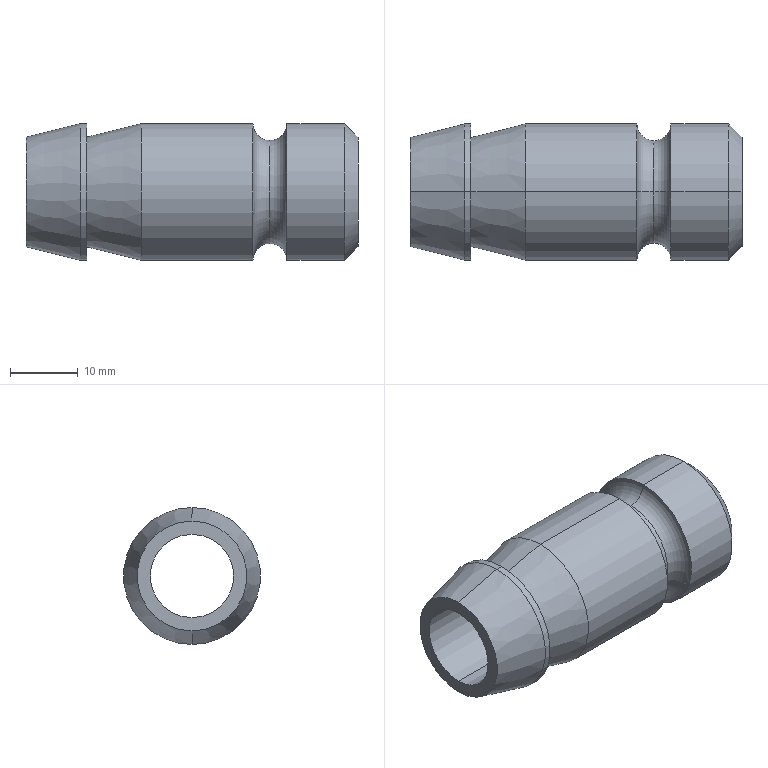Part | SolidWorks | features ICE 1, Revolution 1 | 1 solid | 21 faces | box 49 x 20.2 x 20.2 mm | volume 8256 mm3 | cylinder 8 | cone 6 | torus 4 | plane 3 | commonest cylinder face diameters 20.2 x6 12.3 x2
STEP:
#1=CARTESIAN_POINT('',(33.5,0.,10.1));
#2=VERTEX_POINT('',#1);
#3=CARTESIAN_POINT('',(36.,0.,7.6));
#4=VERTEX_POINT('',#3);
#5=CARTESIAN_POINT('',(36.,0.,10.1));
#6=DIRECTION('',(0.,-1.,0.));
#7=DIRECTION('',(0.,0.,-1.));
#8=AXIS2_PLACEMENT_3D('',#5,#6,#7);
#9=CIRCLE('',#8,2.5);
#10=EDGE_CURVE('',#2,#4,#9,.T.);
#11=ORIENTED_EDGE('',*,*,#10,.T.);
#12=CARTESIAN_POINT('',(36.,0.,-7.6));
#13=VERTEX_POINT('',#12);
#14=CARTESIAN_POINT('',(36.,0.,0.));
#15=DIRECTION('',(-1.,0.,0.));
#16=DIRECTION('',(0.,0.,1.));
#17=AXIS2_PLACEMENT_3D('',#14,#15,#16);
#18=CIRCLE('',#17,7.6);
#19=EDGE_CURVE('',#4,#13,#18,.T.);
#20=ORIENTED_EDGE('',*,*,#19,.T.);
#21=CARTESIAN_POINT('',(33.5,0.,-10.1));
#22=VERTEX_POINT('',#21);
#23=CARTESIAN_POINT('',(36.,0.,-10.1));
#24=DIRECTION('',(0.,1.,0.));
#25=DIRECTION('',(0.,0.,1.));
#26=AXIS2_PLACEMENT_3D('',#23,#24,#25);
#27=CIRCLE('',#26,2.5);
#28=EDGE_CURVE('',#22,#13,#27,.T.);
#29=ORIENTED_EDGE('',*,*,#28,.F.);
#30=CARTESIAN_POINT('',(33.5,0.,0.));
#31=DIRECTION('',(-1.,0.,0.));
#32=DIRECTION('',(0.,0.,1.));
#33=AXIS2_PLACEMENT_3D('',#30,#31,#32);
#34=CIRCLE('',#33,10.1);
#35=EDGE_CURVE('',#2,#22,#34,.T.);
#36=ORIENTED_EDGE('',*,*,#35,.F.);
#37=EDGE_LOOP('',(#11,#20,#29,#36));
#38=FACE_OUTER_BOUND('',#37,.T.);
#39=CARTESIAN_POINT('',(36.,0.,0.));
#40=DIRECTION('',(-1.,0.,0.));
#41=DIRECTION('',(0.,0.,1.));
#42=AXIS2_PLACEMENT_3D('',#39,#40,#41);
#43=TOROIDAL_SURFACE('',#42,10.1,2.5);
#44=ADVANCED_FACE('',(#38),#43,.F.);
#45=ORIENTED_EDGE('',*,*,#28,.T.);
#46=CARTESIAN_POINT('',(36.,0.,0.));
#47=DIRECTION('',(-1.,0.,0.));
#48=DIRECTION('',(0.,0.,1.));
#49=AXIS2_PLACEMENT_3D('',#46,#47,#48);
#50=CIRCLE('',#49,7.6);
#51=EDGE_CURVE('',#13,#4,#50,.T.);
#52=ORIENTED_EDGE('',*,*,#51,.T.);
#53=ORIENTED_EDGE('',*,*,#10,.F.);
#54=CARTESIAN_POINT('',(33.5,0.,0.));
#55=DIRECTION('',(-1.,0.,0.));
#56=DIRECTION('',(0.,0.,1.));
#57=AXIS2_PLACEMENT_3D('',#54,#55,#56);
#58=CIRCLE('',#57,10.1);
#59=EDGE_CURVE('',#22,#2,#58,.T.);
#60=ORIENTED_EDGE('',*,*,#59,.F.);
#61=EDGE_LOOP('',(#45,#52,#53,#60));
#62=FACE_OUTER_BOUND('',#61,.T.);
#63=CARTESIAN_POINT('',(36.,0.,0.));
#64=DIRECTION('',(-1.,0.,0.));
#65=DIRECTION('',(0.,0.,1.));
#66=AXIS2_PLACEMENT_3D('',#63,#64,#65);
#67=TOROIDAL_SURFACE('',#66,10.1,2.5);
#68=ADVANCED_FACE('',(#62),#67,.F.);
#69=CARTESIAN_POINT('',(49.,0.,-6.15));
#70=VERTEX_POINT('',#69);
#71=CARTESIAN_POINT('',(49.,0.,6.15));
#72=VERTEX_POINT('',#71);
#73=CARTESIAN_POINT('',(49.,0.,0.));
#74=DIRECTION('',(-1.,0.,0.));
#75=DIRECTION('',(0.,0.,1.));
#76=AXIS2_PLACEMENT_3D('',#73,#74,#75);
#77=CIRCLE('',#76,6.15);
#78=EDGE_CURVE('',#70,#72,#77,.T.);
#79=ORIENTED_EDGE('',*,*,#78,.F.);
#80=CARTESIAN_POINT('',(0.,0.,-6.15));
#81=VERTEX_POINT('',#80);
#82=CARTESIAN_POINT('',(99.,0.,-6.15));
#83=DIRECTION('',(-1.,0.,0.));
#84=VECTOR('',#83,1000.);
#85=LINE('',#82,#84);
#86=EDGE_CURVE('',#70,#81,#85,.T.);
#87=ORIENTED_EDGE('',*,*,#86,.T.);
#88=CARTESIAN_POINT('',(0.,0.,6.15));
#89=VERTEX_POINT('',#88);
#90=CARTESIAN_POINT('',(0.,0.,0.));
#91=DIRECTION('',(-1.,0.,0.));
#92=DIRECTION('',(0.,0.,1.));
#93=AXIS2_PLACEMENT_3D('',#90,#91,#92);
#94=CIRCLE('',#93,6.15);
#95=EDGE_CURVE('',#81,#89,#94,.T.);
#96=ORIENTED_EDGE('',*,*,#95,.T.);
#97=CARTESIAN_POINT('',(99.,0.,6.15));
#98=DIRECTION('',(-1.,0.,0.));
#99=VECTOR('',#98,1000.);
#100=LINE('',#97,#99);
#101=EDGE_CURVE('',#72,#89,#100,.T.);
#102=ORIENTED_EDGE('',*,*,#101,.F.);
#103=EDGE_LOOP('',(#79,#87,#96,#102));
#104=FACE_OUTER_BOUND('',#103,.T.);
#105=CARTESIAN_POINT('',(99.,0.,0.));
#106=DIRECTION('',(-1.,0.,0.));
#107=DIRECTION('',(0.,0.,1.));
#108=AXIS2_PLACEMENT_3D('',#105,#106,#107);
#109=CYLINDRICAL_SURFACE('',#108,6.15);
#110=ADVANCED_FACE('',(#104),#109,.F.);
#111=ORIENTED_EDGE('',*,*,#51,.F.);
#112=CARTESIAN_POINT('',(38.5,0.,-10.1));
#113=VERTEX_POINT('',#112);
#114=CARTESIAN_POINT('',(36.,0.,-10.1));
#115=DIRECTION('',(0.,1.,0.));
#116=DIRECTION('',(0.,0.,1.));
#117=AXIS2_PLACEMENT_3D('',#114,#115,#116);
#118=CIRCLE('',#117,2.5);
#119=EDGE_CURVE('',#13,#113,#118,.T.);
#120=ORIENTED_EDGE('',*,*,#119,.T.);
#121=CARTESIAN_POINT('',(38.5,0.,10.1));
#122=VERTEX_POINT('',#121);
#123=CARTESIAN_POINT('',(38.5,0.,0.));
#124=DIRECTION('',(-1.,0.,0.));
#125=DIRECTION('',(0.,0.,1.));
#126=AXIS2_PLACEMENT_3D('',#123,#124,#125);
#127=CIRCLE('',#126,10.1);
#128=EDGE_CURVE('',#113,#122,#127,.T.);
#129=ORIENTED_EDGE('',*,*,#128,.T.);
#130=CARTESIAN_POINT('',(36.,0.,10.1));
#131=DIRECTION('',(0.,-1.,0.));
#132=DIRECTION('',(0.,0.,-1.));
#133=AXIS2_PLACEMENT_3D('',#130,#131,#132);
#134=CIRCLE('',#133,2.5);
#135=EDGE_CURVE('',#4,#122,#134,.T.);
#136=ORIENTED_EDGE('',*,*,#135,.F.);
#137=EDGE_LOOP('',(#111,#120,#129,#136));
#138=FACE_OUTER_BOUND('',#137,.T.);
#139=CARTESIAN_POINT('',(36.,0.,0.));
#140=DIRECTION('',(-1.,0.,0.));
#141=DIRECTION('',(0.,0.,1.));
#142=AXIS2_PLACEMENT_3D('',#139,#140,#141);
#143=TOROIDAL_SURFACE('',#142,10.1,2.5);
#144=ADVANCED_FACE('',(#138),#143,.F.);
#145=CARTESIAN_POINT('',(47.,0.,10.1));
#146=VERTEX_POINT('',#145);
#147=CARTESIAN_POINT('',(47.,0.,-10.1));
#148=VERTEX_POINT('',#147);
#149=CARTESIAN_POINT('',(47.,0.,0.));
#150=DIRECTION('',(-1.,0.,0.));
#151=DIRECTION('',(0.,0.,1.));
#152=AXIS2_PLACEMENT_3D('',#149,#150,#151);
#153=CIRCLE('',#152,10.1);
#154=EDGE_CURVE('',#146,#148,#153,.T.);
#155=ORIENTED_EDGE('',*,*,#154,.T.);
#156=CARTESIAN_POINT('',(0.,0.,-10.1));
#157=DIRECTION('',(-1.,0.,0.));
#158=VECTOR('',#157,1000.);
#159=LINE('',#156,#158);
#160=EDGE_CURVE('',#148,#113,#159,.T.);
#161=ORIENTED_EDGE('',*,*,#160,.T.);
#162=CARTESIAN_POINT('',(38.5,0.,0.));
#163=DIRECTION('',(-1.,0.,0.));
#164=DIRECTION('',(0.,0.,1.));
#165=AXIS2_PLACEMENT_3D('',#162,#163,#164);
#166=CIRCLE('',#165,10.1);
#167=EDGE_CURVE('',#122,#113,#166,.T.);
#168=ORIENTED_EDGE('',*,*,#167,.F.);
#169=CARTESIAN_POINT('',(0.,0.,10.1));
#170=DIRECTION('',(-1.,0.,0.));
#171=VECTOR('',#170,1000.);
#172=LINE('',#169,#171);
#173=EDGE_CURVE('',#146,#122,#172,.T.);
#174=ORIENTED_EDGE('',*,*,#173,.F.);
#175=EDGE_LOOP('',(#155,#161,#168,#174));
#176=FACE_OUTER_BOUND('',#175,.T.);
#177=CARTESIAN_POINT('',(0.,0.,0.));
#178=DIRECTION('',(-1.,0.,0.));
#179=DIRECTION('',(0.,0.,1.));
#180=AXIS2_PLACEMENT_3D('',#177,#178,#179);
#181=CYLINDRICAL_SURFACE('',#180,10.1);
#182=ADVANCED_FACE('',(#176),#181,.T.);
#183=CARTESIAN_POINT('',(49.,0.,8.1));
#184=VERTEX_POINT('',#183);
#185=CARTESIAN_POINT('',(49.,0.,-8.1));
#186=VERTEX_POINT('',#185);
#187=CARTESIAN_POINT('',(49.,0.,0.));
#188=DIRECTION('',(-1.,0.,0.));
#189=DIRECTION('',(0.,0.,1.));
#190=AXIS2_PLACEMENT_3D('',#187,#188,#189);
#191=CIRCLE('',#190,8.1);
#192=EDGE_CURVE('',#184,#186,#191,.T.);
#193=ORIENTED_EDGE('',*,*,#192,.T.);
#194=CARTESIAN_POINT('',(49.,0.,-8.1));
#195=DIRECTION('',(-0.7071,0.,-0.7071));
#196=VECTOR('',#195,1000.);
#197=LINE('',#194,#196);
#198=EDGE_CURVE('',#186,#148,#197,.T.);
#199=ORIENTED_EDGE('',*,*,#198,.T.);
#200=ORIENTED_EDGE('',*,*,#154,.F.);
#201=CARTESIAN_POINT('',(49.,0.,8.1));
#202=DIRECTION('',(-0.7071,0.,0.7071));
#203=VECTOR('',#202,1000.);
#204=LINE('',#201,#203);
#205=EDGE_CURVE('',#184,#146,#204,.T.);
#206=ORIENTED_EDGE('',*,*,#205,.F.);
#207=EDGE_LOOP('',(#193,#199,#200,#206));
#208=FACE_OUTER_BOUND('',#207,.T.);
#209=CARTESIAN_POINT('',(49.,0.,0.));
#210=DIRECTION('',(-1.,0.,0.));
#211=DIRECTION('',(0.,0.,1.));
#212=AXIS2_PLACEMENT_3D('',#209,#210,#211);
#213=CONICAL_SURFACE('',#212,8.1,0.7854);
#214=ADVANCED_FACE('',(#208),#213,.T.);
#215=CARTESIAN_POINT('',(0.,0.,8.1));
#216=VERTEX_POINT('',#215);
#217=CARTESIAN_POINT('',(0.,0.,-8.1));
#218=VERTEX_POINT('',#217);
#219=CARTESIAN_POINT('',(0.,0.,0.));
#220=DIRECTION('',(-1.,0.,0.));
#221=DIRECTION('',(0.,0.,1.));
#222=AXIS2_PLACEMENT_3D('',#219,#220,#221);
#223=CIRCLE('',#222,8.1);
#224=EDGE_CURVE('',#216,#218,#223,.T.);
#225=ORIENTED_EDGE('',*,*,#224,.F.);
#226=CARTESIAN_POINT('',(8.,0.,10.1));
#227=VERTEX_POINT('',#226);
#228=CARTESIAN_POINT('',(8.,0.,10.1));
#229=DIRECTION('',(0.9701,0.,0.2425));
#230=VECTOR('',#229,1000.);
#231=LINE('',#228,#230);
#232=EDGE_CURVE('',#216,#227,#231,.T.);
#233=ORIENTED_EDGE('',*,*,#232,.T.);
#234=CARTESIAN_POINT('',(8.,0.,-10.1));
#235=VERTEX_POINT('',#234);
#236=CARTESIAN_POINT('',(8.,0.,0.));
#237=DIRECTION('',(-1.,0.,0.));
#238=DIRECTION('',(0.,0.,1.));
#239=AXIS2_PLACEMENT_3D('',#236,#237,#238);
#240=CIRCLE('',#239,10.1);
#241=EDGE_CURVE('',#227,#235,#240,.T.);
#242=ORIENTED_EDGE('',*,*,#241,.T.);
#243=CARTESIAN_POINT('',(8.,0.,-10.1));
#244=DIRECTION('',(0.9701,0.,-0.2425));
#245=VECTOR('',#244,1000.);
#246=LINE('',#243,#245);
#247=EDGE_CURVE('',#218,#235,#246,.T.);
#248=ORIENTED_EDGE('',*,*,#247,.F.);
#249=EDGE_LOOP('',(#225,#233,#242,#248));
#250=FACE_OUTER_BOUND('',#249,.T.);
#251=CARTESIAN_POINT('',(8.,0.,0.));
#252=DIRECTION('',(1.,0.,0.));
#253=DIRECTION('',(0.,0.,-1.));
#254=AXIS2_PLACEMENT_3D('',#251,#252,#253);
#255=CONICAL_SURFACE('',#254,10.1,0.245);
#256=ADVANCED_FACE('',(#250),#255,.T.);
#257=CARTESIAN_POINT('',(9.,0.,10.1));
#258=VERTEX_POINT('',#257);
#259=CARTESIAN_POINT('',(9.,0.,-10.1));
#260=VERTEX_POINT('',#259);
#261=CARTESIAN_POINT('',(9.,0.,0.));
#262=DIRECTION('',(-1.,0.,0.));
#263=DIRECTION('',(0.,0.,1.));
#264=AXIS2_PLACEMENT_3D('',#261,#262,#263);
#265=CIRCLE('',#264,10.1);
#266=EDGE_CURVE('',#258,#260,#265,.T.);
#267=ORIENTED_EDGE('',*,*,#266,.T.);
#268=CARTESIAN_POINT('',(0.,0.,-10.1));
#269=DIRECTION('',(-1.,0.,0.));
#270=VECTOR('',#269,1000.);
#271=LINE('',#268,#270);
#272=EDGE_CURVE('',#260,#235,#271,.T.);
#273=ORIENTED_EDGE('',*,*,#272,.T.);
#274=ORIENTED_EDGE('',*,*,#241,.F.);
#275=CARTESIAN_POINT('',(0.,0.,10.1));
#276=DIRECTION('',(-1.,0.,0.));
#277=VECTOR('',#276,1000.);
#278=LINE('',#275,#277);
#279=EDGE_CURVE('',#258,#227,#278,.T.);
#280=ORIENTED_EDGE('',*,*,#279,.F.);
#281=EDGE_LOOP('',(#267,#273,#274,#280));
#282=FACE_OUTER_BOUND('',#281,.T.);
#283=CARTESIAN_POINT('',(0.,0.,0.));
#284=DIRECTION('',(-1.,0.,0.));
#285=DIRECTION('',(0.,0.,1.));
#286=AXIS2_PLACEMENT_3D('',#283,#284,#285);
#287=CYLINDRICAL_SURFACE('',#286,10.1);
#288=ADVANCED_FACE('',(#282),#287,.T.);
#289=CARTESIAN_POINT('',(9.,0.,8.1));
#290=VERTEX_POINT('',#289);
#291=CARTESIAN_POINT('',(9.,0.,-8.1));
#292=VERTEX_POINT('',#291);
#293=CARTESIAN_POINT('',(9.,0.,0.));
#294=DIRECTION('',(-1.,0.,0.));
#295=DIRECTION('',(0.,0.,1.));
#296=AXIS2_PLACEMENT_3D('',#293,#294,#295);
#297=CIRCLE('',#296,8.1);
#298=EDGE_CURVE('',#290,#292,#297,.T.);
#299=ORIENTED_EDGE('',*,*,#298,.F.);
#300=CARTESIAN_POINT('',(17.,0.,10.1));
#301=VERTEX_POINT('',#300);
#302=CARTESIAN_POINT('',(17.,0.,10.1));
#303=DIRECTION('',(0.9701,0.,0.2425));
#304=VECTOR('',#303,1000.);
#305=LINE('',#302,#304);
#306=EDGE_CURVE('',#290,#301,#305,.T.);
#307=ORIENTED_EDGE('',*,*,#306,.T.);
#308=CARTESIAN_POINT('',(17.,0.,-10.1));
#309=VERTEX_POINT('',#308);
#310=CARTESIAN_POINT('',(17.,0.,0.));
#311=DIRECTION('',(-1.,0.,0.));
#312=DIRECTION('',(0.,0.,1.));
#313=AXIS2_PLACEMENT_3D('',#310,#311,#312);
#314=CIRCLE('',#313,10.1);
#315=EDGE_CURVE('',#301,#309,#314,.T.);
#316=ORIENTED_EDGE('',*,*,#315,.T.);
#317=CARTESIAN_POINT('',(17.,0.,-10.1));
#318=DIRECTION('',(0.9701,0.,-0.2425));
#319=VECTOR('',#318,1000.);
#320=LINE('',#317,#319);
#321=EDGE_CURVE('',#292,#309,#320,.T.);
#322=ORIENTED_EDGE('',*,*,#321,.F.);
#323=EDGE_LOOP('',(#299,#307,#316,#322));
#324=FACE_OUTER_BOUND('',#323,.T.);
#325=CARTESIAN_POINT('',(17.,0.,0.));
#326=DIRECTION('',(1.,0.,0.));
#327=DIRECTION('',(0.,0.,-1.));
#328=AXIS2_PLACEMENT_3D('',#325,#326,#327);
#329=CONICAL_SURFACE('',#328,10.1,0.245);
#330=ADVANCED_FACE('',(#324),#329,.T.);
#331=ORIENTED_EDGE('',*,*,#35,.T.);
#332=CARTESIAN_POINT('',(0.,0.,-10.1));
#333=DIRECTION('',(-1.,0.,0.));
#334=VECTOR('',#333,1000.);
#335=LINE('',#332,#334);
#336=EDGE_CURVE('',#22,#309,#335,.T.);
#337=ORIENTED_EDGE('',*,*,#336,.T.);
#338=ORIENTED_EDGE('',*,*,#315,.F.);
#339=CARTESIAN_POINT('',(0.,0.,10.1));
#340=DIRECTION('',(-1.,0.,0.));
#341=VECTOR('',#340,1000.);
#342=LINE('',#339,#341);
#343=EDGE_CURVE('',#2,#301,#342,.T.);
#344=ORIENTED_EDGE('',*,*,#343,.F.);
#345=EDGE_LOOP('',(#331,#337,#338,#344));
#346=FACE_OUTER_BOUND('',#345,.T.);
#347=CARTESIAN_POINT('',(0.,0.,0.));
#348=DIRECTION('',(-1.,0.,0.));
#349=DIRECTION('',(0.,0.,1.));
#350=AXIS2_PLACEMENT_3D('',#347,#348,#349);
#351=CYLINDRICAL_SURFACE('',#350,10.1);
#352=ADVANCED_FACE('',(#346),#351,.T.);
#353=ORIENTED_EDGE('',*,*,#336,.F.);
#354=ORIENTED_EDGE('',*,*,#59,.T.);
#355=ORIENTED_EDGE('',*,*,#343,.T.);
#356=CARTESIAN_POINT('',(17.,0.,0.));
#357=DIRECTION('',(-1.,0.,0.));
#358=DIRECTION('',(0.,0.,1.));
#359=AXIS2_PLACEMENT_3D('',#356,#357,#358);
#360=CIRCLE('',#359,10.1);
#361=EDGE_CURVE('',#309,#301,#360,.T.);
#362=ORIENTED_EDGE('',*,*,#361,.F.);
#363=EDGE_LOOP('',(#353,#354,#355,#362));
#364=FACE_OUTER_BOUND('',#363,.T.);
#365=CARTESIAN_POINT('',(0.,0.,0.));
#366=DIRECTION('',(-1.,0.,0.));
#367=DIRECTION('',(0.,0.,1.));
#368=AXIS2_PLACEMENT_3D('',#365,#366,#367);
#369=CYLINDRICAL_SURFACE('',#368,10.1);
#370=ADVANCED_FACE('',(#364),#369,.T.);
#371=ORIENTED_EDGE('',*,*,#306,.F.);
#372=CARTESIAN_POINT('',(9.,0.,0.));
#373=DIRECTION('',(-1.,0.,0.));
#374=DIRECTION('',(0.,0.,1.));
#375=AXIS2_PLACEMENT_3D('',#372,#373,#374);
#376=CIRCLE('',#375,8.1);
#377=EDGE_CURVE('',#292,#290,#376,.T.);
#378=ORIENTED_EDGE('',*,*,#377,.F.);
#379=ORIENTED_EDGE('',*,*,#321,.T.);
#380=ORIENTED_EDGE('',*,*,#361,.T.);
#381=EDGE_LOOP('',(#371,#378,#379,#380));
#382=FACE_OUTER_BOUND('',#381,.T.);
#383=CARTESIAN_POINT('',(17.,0.,0.));
#384=DIRECTION('',(1.,0.,0.));
#385=DIRECTION('',(0.,0.,-1.));
#386=AXIS2_PLACEMENT_3D('',#383,#384,#385);
#387=CONICAL_SURFACE('',#386,10.1,0.245);
#388=ADVANCED_FACE('',(#382),#387,.T.);
#389=ORIENTED_EDGE('',*,*,#266,.F.);
#390=CARTESIAN_POINT('',(9.,0.,0.));
#391=DIRECTION('',(-1.,0.,0.));
#392=DIRECTION('',(0.,0.,1.));
#393=AXIS2_PLACEMENT_3D('',#390,#391,#392);
#394=CIRCLE('',#393,10.1);
#395=EDGE_CURVE('',#260,#258,#394,.T.);
#396=ORIENTED_EDGE('',*,*,#395,.F.);
#397=EDGE_LOOP('',(#389,#396));
#398=FACE_OUTER_BOUND('',#397,.T.);
#399=ORIENTED_EDGE('',*,*,#377,.T.);
#400=ORIENTED_EDGE('',*,*,#298,.T.);
#401=EDGE_LOOP('',(#399,#400));
#402=FACE_BOUND('',#401,.T.);
#403=CARTESIAN_POINT('',(9.,8.1,0.));
#404=DIRECTION('',(-1.,0.,0.));
#405=DIRECTION('',(0.,0.,1.));
#406=AXIS2_PLACEMENT_3D('',#403,#404,#405);
#407=PLANE('',#406);
#408=ADVANCED_FACE('',(#398,#402),#407,.F.);
#409=ORIENTED_EDGE('',*,*,#272,.F.);
#410=ORIENTED_EDGE('',*,*,#395,.T.);
#411=ORIENTED_EDGE('',*,*,#279,.T.);
#412=CARTESIAN_POINT('',(8.,0.,0.));
#413=DIRECTION('',(-1.,0.,0.));
#414=DIRECTION('',(0.,0.,1.));
#415=AXIS2_PLACEMENT_3D('',#412,#413,#414);
#416=CIRCLE('',#415,10.1);
#417=EDGE_CURVE('',#235,#227,#416,.T.);
#418=ORIENTED_EDGE('',*,*,#417,.F.);
#419=EDGE_LOOP('',(#409,#410,#411,#418));
#420=FACE_OUTER_BOUND('',#419,.T.);
#421=CARTESIAN_POINT('',(0.,0.,0.));
#422=DIRECTION('',(-1.,0.,0.));
#423=DIRECTION('',(0.,0.,1.));
#424=AXIS2_PLACEMENT_3D('',#421,#422,#423);
#425=CYLINDRICAL_SURFACE('',#424,10.1);
#426=ADVANCED_FACE('',(#420),#425,.T.);
#427=ORIENTED_EDGE('',*,*,#232,.F.);
#428=CARTESIAN_POINT('',(0.,0.,0.));
#429=DIRECTION('',(-1.,0.,0.));
#430=DIRECTION('',(0.,0.,1.));
#431=AXIS2_PLACEMENT_3D('',#428,#429,#430);
#432=CIRCLE('',#431,8.1);
#433=EDGE_CURVE('',#218,#216,#432,.T.);
#434=ORIENTED_EDGE('',*,*,#433,.F.);
#435=ORIENTED_EDGE('',*,*,#247,.T.);
#436=ORIENTED_EDGE('',*,*,#417,.T.);
#437=EDGE_LOOP('',(#427,#434,#435,#436));
#438=FACE_OUTER_BOUND('',#437,.T.);
#439=CARTESIAN_POINT('',(8.,0.,0.));
#440=DIRECTION('',(1.,0.,0.));
#441=DIRECTION('',(0.,0.,-1.));
#442=AXIS2_PLACEMENT_3D('',#439,#440,#441);
#443=CONICAL_SURFACE('',#442,10.1,0.245);
#444=ADVANCED_FACE('',(#438),#443,.T.);
#445=CARTESIAN_POINT('',(0.,0.,0.));
#446=DIRECTION('',(-1.,0.,0.));
#447=DIRECTION('',(0.,0.,1.));
#448=AXIS2_PLACEMENT_3D('',#445,#446,#447);
#449=CIRCLE('',#448,6.15);
#450=EDGE_CURVE('',#89,#81,#449,.T.);
#451=ORIENTED_EDGE('',*,*,#450,.F.);
#452=ORIENTED_EDGE('',*,*,#95,.F.);
#453=EDGE_LOOP('',(#451,#452));
#454=FACE_BOUND('',#453,.T.);
#455=ORIENTED_EDGE('',*,*,#433,.T.);
#456=ORIENTED_EDGE('',*,*,#224,.T.);
#457=EDGE_LOOP('',(#455,#456));
#458=FACE_OUTER_BOUND('',#457,.T.);
#459=CARTESIAN_POINT('',(0.,8.1,0.));
#460=DIRECTION('',(1.,0.,0.));
#461=DIRECTION('',(0.,0.,-1.));
#462=AXIS2_PLACEMENT_3D('',#459,#460,#461);
#463=PLANE('',#462);
#464=ADVANCED_FACE('',(#454,#458),#463,.F.);
#465=CARTESIAN_POINT('',(49.,0.,0.));
#466=DIRECTION('',(-1.,0.,0.));
#467=DIRECTION('',(0.,0.,1.));
#468=AXIS2_PLACEMENT_3D('',#465,#466,#467);
#469=CIRCLE('',#468,6.15);
#470=EDGE_CURVE('',#72,#70,#469,.T.);
#471=ORIENTED_EDGE('',*,*,#470,.T.);
#472=ORIENTED_EDGE('',*,*,#78,.T.);
#473=EDGE_LOOP('',(#471,#472));
#474=FACE_BOUND('',#473,.T.);
#475=ORIENTED_EDGE('',*,*,#192,.F.);
#476=CARTESIAN_POINT('',(49.,0.,0.));
#477=DIRECTION('',(-1.,0.,0.));
#478=DIRECTION('',(0.,0.,1.));
#479=AXIS2_PLACEMENT_3D('',#476,#477,#478);
#480=CIRCLE('',#479,8.1);
#481=EDGE_CURVE('',#186,#184,#480,.T.);
#482=ORIENTED_EDGE('',*,*,#481,.F.);
#483=EDGE_LOOP('',(#475,#482));
#484=FACE_OUTER_BOUND('',#483,.T.);
#485=CARTESIAN_POINT('',(49.,8.1,0.));
#486=DIRECTION('',(-1.,0.,0.));
#487=DIRECTION('',(0.,0.,1.));
#488=AXIS2_PLACEMENT_3D('',#485,#486,#487);
#489=PLANE('',#488);
#490=ADVANCED_FACE('',(#474,#484),#489,.F.);
#491=ORIENTED_EDGE('',*,*,#198,.F.);
#492=ORIENTED_EDGE('',*,*,#481,.T.);
#493=ORIENTED_EDGE('',*,*,#205,.T.);
#494=CARTESIAN_POINT('',(47.,0.,0.));
#495=DIRECTION('',(-1.,0.,0.));
#496=DIRECTION('',(0.,0.,1.));
#497=AXIS2_PLACEMENT_3D('',#494,#495,#496);
#498=CIRCLE('',#497,10.1);
#499=EDGE_CURVE('',#148,#146,#498,.T.);
#500=ORIENTED_EDGE('',*,*,#499,.F.);
#501=EDGE_LOOP('',(#491,#492,#493,#500));
#502=FACE_OUTER_BOUND('',#501,.T.);
#503=CARTESIAN_POINT('',(49.,0.,0.));
#504=DIRECTION('',(-1.,0.,0.));
#505=DIRECTION('',(0.,0.,1.));
#506=AXIS2_PLACEMENT_3D('',#503,#504,#505);
#507=CONICAL_SURFACE('',#506,8.1,0.7854);
#508=ADVANCED_FACE('',(#502),#507,.T.);
#509=ORIENTED_EDGE('',*,*,#160,.F.);
#510=ORIENTED_EDGE('',*,*,#499,.T.);
#511=ORIENTED_EDGE('',*,*,#173,.T.);
#512=ORIENTED_EDGE('',*,*,#128,.F.);
#513=EDGE_LOOP('',(#509,#510,#511,#512));
#514=FACE_OUTER_BOUND('',#513,.T.);
#515=CARTESIAN_POINT('',(0.,0.,0.));
#516=DIRECTION('',(-1.,0.,0.));
#517=DIRECTION('',(0.,0.,1.));
#518=AXIS2_PLACEMENT_3D('',#515,#516,#517);
#519=CYLINDRICAL_SURFACE('',#518,10.1);
#520=ADVANCED_FACE('',(#514),#519,.T.);
#521=ORIENTED_EDGE('',*,*,#19,.F.);
#522=ORIENTED_EDGE('',*,*,#135,.T.);
#523=ORIENTED_EDGE('',*,*,#167,.T.);
#524=ORIENTED_EDGE('',*,*,#119,.F.);
#525=EDGE_LOOP('',(#521,#522,#523,#524));
#526=FACE_OUTER_BOUND('',#525,.T.);
#527=CARTESIAN_POINT('',(36.,0.,0.));
#528=DIRECTION('',(-1.,0.,0.));
#529=DIRECTION('',(0.,0.,1.));
#530=AXIS2_PLACEMENT_3D('',#527,#528,#529);
#531=TOROIDAL_SURFACE('',#530,10.1,2.5);
#532=ADVANCED_FACE('',(#526),#531,.F.);
#533=ORIENTED_EDGE('',*,*,#86,.F.);
#534=ORIENTED_EDGE('',*,*,#470,.F.);
#535=ORIENTED_EDGE('',*,*,#101,.T.);
#536=ORIENTED_EDGE('',*,*,#450,.T.);
#537=EDGE_LOOP('',(#533,#534,#535,#536));
#538=FACE_OUTER_BOUND('',#537,.T.);
#539=CARTESIAN_POINT('',(99.,0.,0.));
#540=DIRECTION('',(-1.,0.,0.));
#541=DIRECTION('',(0.,0.,1.));
#542=AXIS2_PLACEMENT_3D('',#539,#540,#541);
#543=CYLINDRICAL_SURFACE('',#542,6.15);
#544=ADVANCED_FACE('',(#538),#543,.F.);
#545=CLOSED_SHELL('',(#44,#68,#110,#144,#182,#214,#256,#288,#330,#352,#370,#388,#408,#426,#444,#464,#490,#508,#520,#532,#544));
#546=MANIFOLD_SOLID_BREP('',#545);
#547=CARTESIAN_POINT('',(0.,0.,0.));
#548=DIRECTION('',(0.,0.,1.));
#549=DIRECTION('',(1.,0.,0.));
#550=AXIS2_PLACEMENT_3D('',#547,#548,#549);
#551=(LENGTH_UNIT()NAMED_UNIT(*)SI_UNIT(.MILLI.,.METRE.));
#552=UNCERTAINTY_MEASURE_WITH_UNIT(LENGTH_MEASURE(0.00001),#551,'','');
#553=(NAMED_UNIT(*)PLANE_ANGLE_UNIT()SI_UNIT($,.RADIAN.));
#554=(NAMED_UNIT(*)SI_UNIT($,.STERADIAN.)SOLID_ANGLE_UNIT());
#555=(GEOMETRIC_REPRESENTATION_CONTEXT(3)GLOBAL_UNCERTAINTY_ASSIGNED_CONTEXT((#552))GLOBAL_UNIT_ASSIGNED_CONTEXT((#551,#553,#554))REPRESENTATION_CONTEXT('',''));
#556=ADVANCED_BREP_SHAPE_REPRESENTATION('',(#546,#550),#555);